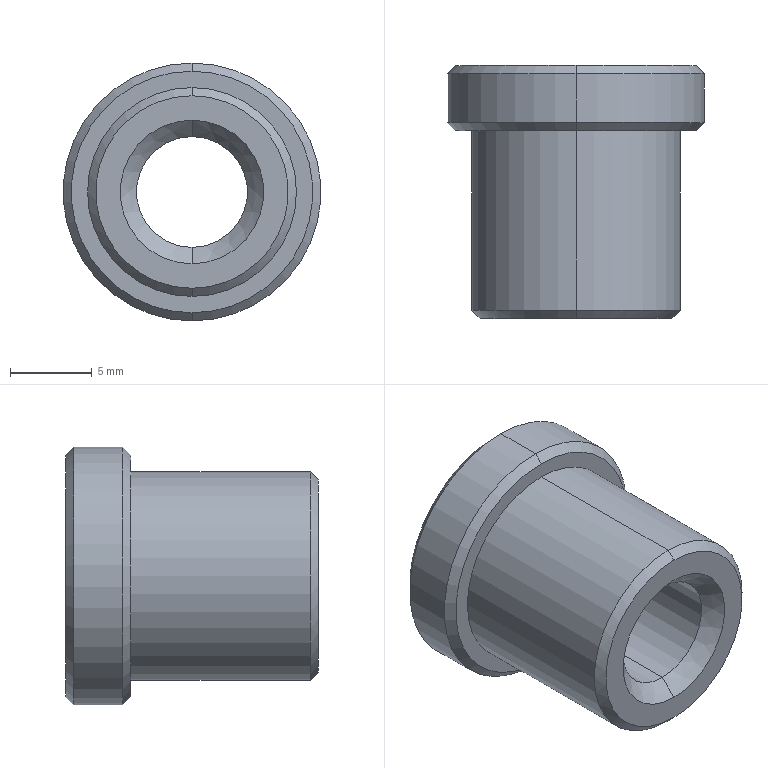Part | STEP file | CA-10-019Floating Joint | 1 solid | 19 faces | box 15.8 x 15.5 x 15.8 mm | volume 1661 mm3 | cone 10 | cylinder 6 | plane 3 | commonest cylinder face diameters 6.8 x2 12.8 x2 15.8 x2
STEP:
#1=CARTESIAN_POINT('',(0.,0.,0.));
#2=DIRECTION('',(0.,0.,1.));
#3=DIRECTION('',(1.,0.,0.));
#4=AXIS2_PLACEMENT_3D('',#1,#2,#3);
#5=CARTESIAN_POINT('',(0.,0.,-5.9));
#6=VERTEX_POINT('',#5);
#7=CARTESIAN_POINT('',(0.,0.,5.9));
#8=VERTEX_POINT('',#7);
#9=CARTESIAN_POINT('',(0.,0.,0.));
#10=DIRECTION('',(0.,-1.,0.));
#11=DIRECTION('',(0.,0.,-1.));
#12=AXIS2_PLACEMENT_3D('',#9,#10,#11);
#13=CIRCLE('',#12,5.9);
#14=CARTESIAN_POINT('',(0.,0.5,0.));
#15=DIRECTION('',(0.,1.,0.));
#16=DIRECTION('',(0.,0.,1.));
#17=AXIS2_PLACEMENT_3D('',#14,#15,#16);
#18=CONICAL_SURFACE('',#17,6.4,0.7854);
#19=CARTESIAN_POINT('',(3.142,-0.5));
#20=DIRECTION('',(-1.,0.));
#21=VECTOR('',#20,1.);
#22=LINE('',#19,#21);
#23=(GEOMETRIC_REPRESENTATION_CONTEXT(2)PARAMETRIC_REPRESENTATION_CONTEXT()REPRESENTATION_CONTEXT('',''));
#24=DEFINITIONAL_REPRESENTATION('',(#22),#23);
#25=PCURVE('',#18,#24);
#26=CARTESIAN_POINT('',(-2.5,0.,0.));
#27=DIRECTION('',(0.,-1.,0.));
#28=DIRECTION('',(0.,0.,-1.));
#29=AXIS2_PLACEMENT_3D('',#26,#27,#28);
#30=PLANE('',#29);
#31=CARTESIAN_POINT('',(0.,2.5));
#32=DIRECTION('',(1.,0.));
#33=AXIS2_PLACEMENT_2D('',#31,#32);
#34=CIRCLE('',#33,5.9);
#35=(GEOMETRIC_REPRESENTATION_CONTEXT(2)PARAMETRIC_REPRESENTATION_CONTEXT()REPRESENTATION_CONTEXT('',''));
#36=DEFINITIONAL_REPRESENTATION('',(#34),#35);
#37=PCURVE('',#30,#36);
#38=SURFACE_CURVE('',#13,(#25,#37),.PCURVE_S1.);
#39=EDGE_CURVE('',#6,#8,#38,.T.);
#40=ORIENTED_EDGE('',*,*,#39,.F.);
#41=CARTESIAN_POINT('',(0.,0.5,-6.4));
#42=VERTEX_POINT('',#41);
#43=CARTESIAN_POINT('',(0.,0.5,-6.4));
#44=DIRECTION('',(0.,0.7071,-0.7071));
#45=VECTOR('',#44,1.);
#46=LINE('',#43,#45);
#47=CARTESIAN_POINT('',(3.142,0.));
#48=DIRECTION('',(0.,1.));
#49=VECTOR('',#48,1.);
#50=LINE('',#47,#49);
#51=(GEOMETRIC_REPRESENTATION_CONTEXT(2)PARAMETRIC_REPRESENTATION_CONTEXT()REPRESENTATION_CONTEXT('',''));
#52=DEFINITIONAL_REPRESENTATION('',(#50),#51);
#53=PCURVE('',#18,#52);
#54=CARTESIAN_POINT('',(0.,0.5,0.));
#55=DIRECTION('',(0.,1.,0.));
#56=DIRECTION('',(0.,0.,1.));
#57=AXIS2_PLACEMENT_3D('',#54,#55,#56);
#58=CONICAL_SURFACE('',#57,6.4,0.7854);
#59=CARTESIAN_POINT('',(3.142,0.));
#60=DIRECTION('',(0.,1.));
#61=VECTOR('',#60,1.);
#62=LINE('',#59,#61);
#63=(GEOMETRIC_REPRESENTATION_CONTEXT(2)PARAMETRIC_REPRESENTATION_CONTEXT()REPRESENTATION_CONTEXT('',''));
#64=DEFINITIONAL_REPRESENTATION('',(#62),#63);
#65=PCURVE('',#58,#64);
#66=SURFACE_CURVE('',#46,(#53,#65),.PCURVE_S1.);
#67=EDGE_CURVE('',#6,#42,#66,.T.);
#68=ORIENTED_EDGE('',*,*,#67,.T.);
#69=CARTESIAN_POINT('',(0.,0.5,6.4));
#70=VERTEX_POINT('',#69);
#71=CARTESIAN_POINT('',(0.,0.5,0.));
#72=DIRECTION('',(0.,1.,0.));
#73=DIRECTION('',(0.,0.,-1.));
#74=AXIS2_PLACEMENT_3D('',#71,#72,#73);
#75=CIRCLE('',#74,6.4);
#76=CARTESIAN_POINT('',(-3.142,0.));
#77=DIRECTION('',(1.,0.));
#78=VECTOR('',#77,1.);
#79=LINE('',#76,#78);
#80=(GEOMETRIC_REPRESENTATION_CONTEXT(2)PARAMETRIC_REPRESENTATION_CONTEXT()REPRESENTATION_CONTEXT('',''));
#81=DEFINITIONAL_REPRESENTATION('',(#79),#80);
#82=PCURVE('',#18,#81);
#83=CARTESIAN_POINT('',(0.,-2.167,0.));
#84=DIRECTION('',(0.,1.,0.));
#85=DIRECTION('',(0.,0.,1.));
#86=AXIS2_PLACEMENT_3D('',#83,#84,#85);
#87=CYLINDRICAL_SURFACE('',#86,6.4);
#88=CARTESIAN_POINT('',(-3.142,2.667));
#89=DIRECTION('',(1.,0.));
#90=VECTOR('',#89,1.);
#91=LINE('',#88,#90);
#92=(GEOMETRIC_REPRESENTATION_CONTEXT(2)PARAMETRIC_REPRESENTATION_CONTEXT()REPRESENTATION_CONTEXT('',''));
#93=DEFINITIONAL_REPRESENTATION('',(#91),#92);
#94=PCURVE('',#87,#93);
#95=SURFACE_CURVE('',#75,(#82,#94),.PCURVE_S1.);
#96=EDGE_CURVE('',#70,#42,#95,.T.);
#97=ORIENTED_EDGE('',*,*,#96,.F.);
#98=CARTESIAN_POINT('',(0.,0.5,6.4));
#99=DIRECTION('',(0.,0.7071,0.7071));
#100=VECTOR('',#99,1.);
#101=LINE('',#98,#100);
#102=CARTESIAN_POINT('',(0.,0.));
#103=DIRECTION('',(0.,1.));
#104=VECTOR('',#103,1.);
#105=LINE('',#102,#104);
#106=(GEOMETRIC_REPRESENTATION_CONTEXT(2)PARAMETRIC_REPRESENTATION_CONTEXT()REPRESENTATION_CONTEXT('',''));
#107=DEFINITIONAL_REPRESENTATION('',(#105),#106);
#108=PCURVE('',#18,#107);
#109=CARTESIAN_POINT('',(6.283,0.));
#110=DIRECTION('',(0.,1.));
#111=VECTOR('',#110,1.);
#112=LINE('',#109,#111);
#113=(GEOMETRIC_REPRESENTATION_CONTEXT(2)PARAMETRIC_REPRESENTATION_CONTEXT()REPRESENTATION_CONTEXT('',''));
#114=DEFINITIONAL_REPRESENTATION('',(#112),#113);
#115=PCURVE('',#58,#114);
#116=SURFACE_CURVE('',#101,(#108,#115),.PCURVE_S1.);
#117=EDGE_CURVE('',#8,#70,#116,.T.);
#118=ORIENTED_EDGE('',*,*,#117,.F.);
#119=EDGE_LOOP('',(#40,#68,#97,#118));
#120=FACE_BOUND('',#119,.T.);
#121=ADVANCED_FACE('',(#120),#18,.T.);
#122=CARTESIAN_POINT('',(0.,11.5,-7.4));
#123=VERTEX_POINT('',#122);
#124=CARTESIAN_POINT('',(0.,11.5,7.4));
#125=VERTEX_POINT('',#124);
#126=CARTESIAN_POINT('',(0.,11.5,0.));
#127=DIRECTION('',(0.,-1.,0.));
#128=DIRECTION('',(0.,0.,-1.));
#129=AXIS2_PLACEMENT_3D('',#126,#127,#128);
#130=CIRCLE('',#129,7.4);
#131=CARTESIAN_POINT('',(0.,12.,0.));
#132=DIRECTION('',(0.,1.,0.));
#133=DIRECTION('',(0.,0.,1.));
#134=AXIS2_PLACEMENT_3D('',#131,#132,#133);
#135=CONICAL_SURFACE('',#134,7.9,0.7854);
#136=CARTESIAN_POINT('',(3.142,-0.5));
#137=DIRECTION('',(-1.,0.));
#138=VECTOR('',#137,1.);
#139=LINE('',#136,#138);
#140=(GEOMETRIC_REPRESENTATION_CONTEXT(2)PARAMETRIC_REPRESENTATION_CONTEXT()REPRESENTATION_CONTEXT('',''));
#141=DEFINITIONAL_REPRESENTATION('',(#139),#140);
#142=PCURVE('',#135,#141);
#143=CARTESIAN_POINT('',(-6.4,11.5,0.));
#144=DIRECTION('',(0.,-1.,0.));
#145=DIRECTION('',(0.,0.,-1.));
#146=AXIS2_PLACEMENT_3D('',#143,#144,#145);
#147=PLANE('',#146);
#148=CARTESIAN_POINT('',(0.,6.4));
#149=DIRECTION('',(1.,0.));
#150=AXIS2_PLACEMENT_2D('',#148,#149);
#151=CIRCLE('',#150,7.4);
#152=(GEOMETRIC_REPRESENTATION_CONTEXT(2)PARAMETRIC_REPRESENTATION_CONTEXT()REPRESENTATION_CONTEXT('',''));
#153=DEFINITIONAL_REPRESENTATION('',(#151),#152);
#154=PCURVE('',#147,#153);
#155=SURFACE_CURVE('',#130,(#142,#154),.PCURVE_S1.);
#156=EDGE_CURVE('',#123,#125,#155,.T.);
#157=ORIENTED_EDGE('',*,*,#156,.F.);
#158=CARTESIAN_POINT('',(0.,12.,-7.9));
#159=VERTEX_POINT('',#158);
#160=CARTESIAN_POINT('',(0.,12.,-7.9));
#161=DIRECTION('',(0.,0.7071,-0.7071));
#162=VECTOR('',#161,1.);
#163=LINE('',#160,#162);
#164=CARTESIAN_POINT('',(3.142,0.));
#165=DIRECTION('',(0.,1.));
#166=VECTOR('',#165,1.);
#167=LINE('',#164,#166);
#168=(GEOMETRIC_REPRESENTATION_CONTEXT(2)PARAMETRIC_REPRESENTATION_CONTEXT()REPRESENTATION_CONTEXT('',''));
#169=DEFINITIONAL_REPRESENTATION('',(#167),#168);
#170=PCURVE('',#135,#169);
#171=CARTESIAN_POINT('',(0.,12.,0.));
#172=DIRECTION('',(0.,1.,0.));
#173=DIRECTION('',(0.,0.,1.));
#174=AXIS2_PLACEMENT_3D('',#171,#172,#173);
#175=CONICAL_SURFACE('',#174,7.9,0.7854);
#176=CARTESIAN_POINT('',(3.142,0.));
#177=DIRECTION('',(0.,1.));
#178=VECTOR('',#177,1.);
#179=LINE('',#176,#178);
#180=(GEOMETRIC_REPRESENTATION_CONTEXT(2)PARAMETRIC_REPRESENTATION_CONTEXT()REPRESENTATION_CONTEXT('',''));
#181=DEFINITIONAL_REPRESENTATION('',(#179),#180);
#182=PCURVE('',#175,#181);
#183=SURFACE_CURVE('',#163,(#170,#182),.PCURVE_S1.);
#184=EDGE_CURVE('',#123,#159,#183,.T.);
#185=ORIENTED_EDGE('',*,*,#184,.T.);
#186=CARTESIAN_POINT('',(0.,12.,7.9));
#187=VERTEX_POINT('',#186);
#188=CARTESIAN_POINT('',(0.,12.,0.));
#189=DIRECTION('',(0.,1.,0.));
#190=DIRECTION('',(0.,0.,-1.));
#191=AXIS2_PLACEMENT_3D('',#188,#189,#190);
#192=CIRCLE('',#191,7.9);
#193=CARTESIAN_POINT('',(-3.142,0.));
#194=DIRECTION('',(1.,0.));
#195=VECTOR('',#194,1.);
#196=LINE('',#193,#195);
#197=(GEOMETRIC_REPRESENTATION_CONTEXT(2)PARAMETRIC_REPRESENTATION_CONTEXT()REPRESENTATION_CONTEXT('',''));
#198=DEFINITIONAL_REPRESENTATION('',(#196),#197);
#199=PCURVE('',#135,#198);
#200=CARTESIAN_POINT('',(0.,-2.167,0.));
#201=DIRECTION('',(0.,1.,0.));
#202=DIRECTION('',(0.,0.,1.));
#203=AXIS2_PLACEMENT_3D('',#200,#201,#202);
#204=CYLINDRICAL_SURFACE('',#203,7.9);
#205=CARTESIAN_POINT('',(-3.142,14.167));
#206=DIRECTION('',(1.,0.));
#207=VECTOR('',#206,1.);
#208=LINE('',#205,#207);
#209=(GEOMETRIC_REPRESENTATION_CONTEXT(2)PARAMETRIC_REPRESENTATION_CONTEXT()REPRESENTATION_CONTEXT('',''));
#210=DEFINITIONAL_REPRESENTATION('',(#208),#209);
#211=PCURVE('',#204,#210);
#212=SURFACE_CURVE('',#192,(#199,#211),.PCURVE_S1.);
#213=EDGE_CURVE('',#187,#159,#212,.T.);
#214=ORIENTED_EDGE('',*,*,#213,.F.);
#215=CARTESIAN_POINT('',(0.,12.,7.9));
#216=DIRECTION('',(0.,0.7071,0.7071));
#217=VECTOR('',#216,1.);
#218=LINE('',#215,#217);
#219=CARTESIAN_POINT('',(0.,0.));
#220=DIRECTION('',(0.,1.));
#221=VECTOR('',#220,1.);
#222=LINE('',#219,#221);
#223=(GEOMETRIC_REPRESENTATION_CONTEXT(2)PARAMETRIC_REPRESENTATION_CONTEXT()REPRESENTATION_CONTEXT('',''));
#224=DEFINITIONAL_REPRESENTATION('',(#222),#223);
#225=PCURVE('',#135,#224);
#226=CARTESIAN_POINT('',(6.283,0.));
#227=DIRECTION('',(0.,1.));
#228=VECTOR('',#227,1.);
#229=LINE('',#226,#228);
#230=(GEOMETRIC_REPRESENTATION_CONTEXT(2)PARAMETRIC_REPRESENTATION_CONTEXT()REPRESENTATION_CONTEXT('',''));
#231=DEFINITIONAL_REPRESENTATION('',(#229),#230);
#232=PCURVE('',#175,#231);
#233=SURFACE_CURVE('',#218,(#225,#232),.PCURVE_S1.);
#234=EDGE_CURVE('',#125,#187,#233,.T.);
#235=ORIENTED_EDGE('',*,*,#234,.F.);
#236=EDGE_LOOP('',(#157,#185,#214,#235));
#237=FACE_BOUND('',#236,.T.);
#238=ADVANCED_FACE('',(#237),#135,.T.);
#239=CARTESIAN_POINT('',(0.,15.5,7.4));
#240=VERTEX_POINT('',#239);
#241=CARTESIAN_POINT('',(0.,15.5,-7.4));
#242=VERTEX_POINT('',#241);
#243=CARTESIAN_POINT('',(0.,15.5,0.));
#244=DIRECTION('',(0.,1.,0.));
#245=DIRECTION('',(0.,0.,1.));
#246=AXIS2_PLACEMENT_3D('',#243,#244,#245);
#247=CIRCLE('',#246,7.4);
#248=CARTESIAN_POINT('',(0.,15.5,0.));
#249=DIRECTION('',(0.,-1.,0.));
#250=DIRECTION('',(0.,0.,-1.));
#251=AXIS2_PLACEMENT_3D('',#248,#249,#250);
#252=CONICAL_SURFACE('',#251,7.4,0.7854);
#253=CARTESIAN_POINT('',(3.142,0.));
#254=DIRECTION('',(-1.,0.));
#255=VECTOR('',#254,1.);
#256=LINE('',#253,#255);
#257=(GEOMETRIC_REPRESENTATION_CONTEXT(2)PARAMETRIC_REPRESENTATION_CONTEXT()REPRESENTATION_CONTEXT('',''));
#258=DEFINITIONAL_REPRESENTATION('',(#256),#257);
#259=PCURVE('',#252,#258);
#260=CARTESIAN_POINT('',(-7.9,15.5,0.));
#261=DIRECTION('',(0.,1.,0.));
#262=DIRECTION('',(0.,0.,1.));
#263=AXIS2_PLACEMENT_3D('',#260,#261,#262);
#264=PLANE('',#263);
#265=CARTESIAN_POINT('',(0.,7.9));
#266=DIRECTION('',(1.,0.));
#267=AXIS2_PLACEMENT_2D('',#265,#266);
#268=CIRCLE('',#267,7.4);
#269=(GEOMETRIC_REPRESENTATION_CONTEXT(2)PARAMETRIC_REPRESENTATION_CONTEXT()REPRESENTATION_CONTEXT('',''));
#270=DEFINITIONAL_REPRESENTATION('',(#268),#269);
#271=PCURVE('',#264,#270);
#272=SURFACE_CURVE('',#247,(#259,#271),.PCURVE_S1.);
#273=EDGE_CURVE('',#240,#242,#272,.T.);
#274=ORIENTED_EDGE('',*,*,#273,.F.);
#275=CARTESIAN_POINT('',(0.,15.,7.9));
#276=VERTEX_POINT('',#275);
#277=CARTESIAN_POINT('',(0.,15.5,7.4));
#278=DIRECTION('',(0.,-0.7071,0.7071));
#279=VECTOR('',#278,1.);
#280=LINE('',#277,#279);
#281=CARTESIAN_POINT('',(3.142,0.));
#282=DIRECTION('',(0.,1.));
#283=VECTOR('',#282,1.);
#284=LINE('',#281,#283);
#285=(GEOMETRIC_REPRESENTATION_CONTEXT(2)PARAMETRIC_REPRESENTATION_CONTEXT()REPRESENTATION_CONTEXT('',''));
#286=DEFINITIONAL_REPRESENTATION('',(#284),#285);
#287=PCURVE('',#252,#286);
#288=CARTESIAN_POINT('',(0.,15.5,0.));
#289=DIRECTION('',(0.,-1.,0.));
#290=DIRECTION('',(0.,0.,-1.));
#291=AXIS2_PLACEMENT_3D('',#288,#289,#290);
#292=CONICAL_SURFACE('',#291,7.4,0.7854);
#293=CARTESIAN_POINT('',(3.142,0.));
#294=DIRECTION('',(0.,1.));
#295=VECTOR('',#294,1.);
#296=LINE('',#293,#295);
#297=(GEOMETRIC_REPRESENTATION_CONTEXT(2)PARAMETRIC_REPRESENTATION_CONTEXT()REPRESENTATION_CONTEXT('',''));
#298=DEFINITIONAL_REPRESENTATION('',(#296),#297);
#299=PCURVE('',#292,#298);
#300=SURFACE_CURVE('',#280,(#287,#299),.PCURVE_S1.);
#301=EDGE_CURVE('',#240,#276,#300,.T.);
#302=ORIENTED_EDGE('',*,*,#301,.T.);
#303=CARTESIAN_POINT('',(0.,15.,-7.9));
#304=VERTEX_POINT('',#303);
#305=CARTESIAN_POINT('',(0.,15.,0.));
#306=DIRECTION('',(0.,-1.,0.));
#307=DIRECTION('',(0.,0.,1.));
#308=AXIS2_PLACEMENT_3D('',#305,#306,#307);
#309=CIRCLE('',#308,7.9);
#310=CARTESIAN_POINT('',(-3.142,0.5));
#311=DIRECTION('',(1.,0.));
#312=VECTOR('',#311,1.);
#313=LINE('',#310,#312);
#314=(GEOMETRIC_REPRESENTATION_CONTEXT(2)PARAMETRIC_REPRESENTATION_CONTEXT()REPRESENTATION_CONTEXT('',''));
#315=DEFINITIONAL_REPRESENTATION('',(#313),#314);
#316=PCURVE('',#252,#315);
#317=CARTESIAN_POINT('',(6.283,17.167));
#318=DIRECTION('',(-1.,0.));
#319=VECTOR('',#318,1.);
#320=LINE('',#317,#319);
#321=(GEOMETRIC_REPRESENTATION_CONTEXT(2)PARAMETRIC_REPRESENTATION_CONTEXT()REPRESENTATION_CONTEXT('',''));
#322=DEFINITIONAL_REPRESENTATION('',(#320),#321);
#323=PCURVE('',#204,#322);
#324=SURFACE_CURVE('',#309,(#316,#323),.PCURVE_S1.);
#325=EDGE_CURVE('',#304,#276,#324,.T.);
#326=ORIENTED_EDGE('',*,*,#325,.F.);
#327=CARTESIAN_POINT('',(0.,15.5,-7.4));
#328=DIRECTION('',(0.,-0.7071,-0.7071));
#329=VECTOR('',#328,1.);
#330=LINE('',#327,#329);
#331=CARTESIAN_POINT('',(0.,0.));
#332=DIRECTION('',(0.,1.));
#333=VECTOR('',#332,1.);
#334=LINE('',#331,#333);
#335=(GEOMETRIC_REPRESENTATION_CONTEXT(2)PARAMETRIC_REPRESENTATION_CONTEXT()REPRESENTATION_CONTEXT('',''));
#336=DEFINITIONAL_REPRESENTATION('',(#334),#335);
#337=PCURVE('',#252,#336);
#338=CARTESIAN_POINT('',(6.283,0.));
#339=DIRECTION('',(0.,1.));
#340=VECTOR('',#339,1.);
#341=LINE('',#338,#340);
#342=(GEOMETRIC_REPRESENTATION_CONTEXT(2)PARAMETRIC_REPRESENTATION_CONTEXT()REPRESENTATION_CONTEXT('',''));
#343=DEFINITIONAL_REPRESENTATION('',(#341),#342);
#344=PCURVE('',#292,#343);
#345=SURFACE_CURVE('',#330,(#337,#344),.PCURVE_S1.);
#346=EDGE_CURVE('',#242,#304,#345,.T.);
#347=ORIENTED_EDGE('',*,*,#346,.F.);
#348=EDGE_LOOP('',(#274,#302,#326,#347));
#349=FACE_BOUND('',#348,.T.);
#350=ADVANCED_FACE('',(#349),#252,.T.);
#351=CARTESIAN_POINT('',(0.,14.5,3.4));
#352=VERTEX_POINT('',#351);
#353=CARTESIAN_POINT('',(0.,15.5,4.4));
#354=VERTEX_POINT('',#353);
#355=CARTESIAN_POINT('',(0.,15.5,4.4));
#356=DIRECTION('',(0.,0.7071,0.7071));
#357=VECTOR('',#356,1.);
#358=LINE('',#355,#357);
#359=CARTESIAN_POINT('',(0.,15.5,0.));
#360=DIRECTION('',(0.,1.,0.));
#361=DIRECTION('',(0.,0.,1.));
#362=AXIS2_PLACEMENT_3D('',#359,#360,#361);
#363=CONICAL_SURFACE('',#362,4.4,0.7854);
#364=CARTESIAN_POINT('',(6.283,0.));
#365=DIRECTION('',(0.,1.));
#366=VECTOR('',#365,1.);
#367=LINE('',#364,#366);
#368=(GEOMETRIC_REPRESENTATION_CONTEXT(2)PARAMETRIC_REPRESENTATION_CONTEXT()REPRESENTATION_CONTEXT('',''));
#369=DEFINITIONAL_REPRESENTATION('',(#367),#368);
#370=PCURVE('',#363,#369);
#371=CARTESIAN_POINT('',(0.,15.5,0.));
#372=DIRECTION('',(0.,1.,0.));
#373=DIRECTION('',(0.,0.,1.));
#374=AXIS2_PLACEMENT_3D('',#371,#372,#373);
#375=CONICAL_SURFACE('',#374,4.4,0.7854);
#376=CARTESIAN_POINT('',(0.,0.));
#377=DIRECTION('',(0.,1.));
#378=VECTOR('',#377,1.);
#379=LINE('',#376,#378);
#380=(GEOMETRIC_REPRESENTATION_CONTEXT(2)PARAMETRIC_REPRESENTATION_CONTEXT()REPRESENTATION_CONTEXT('',''));
#381=DEFINITIONAL_REPRESENTATION('',(#379),#380);
#382=PCURVE('',#375,#381);
#383=SURFACE_CURVE('',#358,(#370,#382),.PCURVE_S1.);
#384=EDGE_CURVE('',#352,#354,#383,.T.);
#385=ORIENTED_EDGE('',*,*,#384,.T.);
#386=CARTESIAN_POINT('',(0.,15.5,-4.4));
#387=VERTEX_POINT('',#386);
#388=CARTESIAN_POINT('',(0.,15.5,0.));
#389=DIRECTION('',(0.,-1.,0.));
#390=DIRECTION('',(0.,0.,1.));
#391=AXIS2_PLACEMENT_3D('',#388,#389,#390);
#392=CIRCLE('',#391,4.4);
#393=CARTESIAN_POINT('',(6.283,0.));
#394=DIRECTION('',(-1.,0.));
#395=VECTOR('',#394,1.);
#396=LINE('',#393,#395);
#397=(GEOMETRIC_REPRESENTATION_CONTEXT(2)PARAMETRIC_REPRESENTATION_CONTEXT()REPRESENTATION_CONTEXT('',''));
#398=DEFINITIONAL_REPRESENTATION('',(#396),#397);
#399=PCURVE('',#363,#398);
#400=CARTESIAN_POINT('',(4.4,7.9));
#401=CARTESIAN_POINT('',(4.4,0.279));
#402=CARTESIAN_POINT('',(-2.2,4.089));
#403=CARTESIAN_POINT('',(-8.8,7.9));
#404=CARTESIAN_POINT('',(-2.2,11.711));
#405=CARTESIAN_POINT('',(4.4,15.521));
#406=CARTESIAN_POINT('',(4.4,7.9));
#407=(BOUNDED_CURVE()B_SPLINE_CURVE(2,(#400,#401,#402,#403,#404,#405,#406),.UNSPECIFIED.,.T.,.F.)B_SPLINE_CURVE_WITH_KNOTS((1,2,2,2,2,1),(-2.094,0.,2.094,4.189,6.283,8.378),.UNSPECIFIED.)CURVE()GEOMETRIC_REPRESENTATION_ITEM()RATIONAL_B_SPLINE_CURVE((1.,0.5,1.,0.5,1.,0.5,1.))REPRESENTATION_ITEM(''));
#408=(GEOMETRIC_REPRESENTATION_CONTEXT(2)PARAMETRIC_REPRESENTATION_CONTEXT()REPRESENTATION_CONTEXT('',''));
#409=DEFINITIONAL_REPRESENTATION('',(#407),#408);
#410=PCURVE('',#264,#409);
#411=SURFACE_CURVE('',#392,(#399,#410),.PCURVE_S1.);
#412=EDGE_CURVE('',#354,#387,#411,.T.);
#413=ORIENTED_EDGE('',*,*,#412,.T.);
#414=CARTESIAN_POINT('',(0.,14.5,-3.4));
#415=VERTEX_POINT('',#414);
#416=CARTESIAN_POINT('',(0.,15.5,-4.4));
#417=DIRECTION('',(0.,0.7071,-0.7071));
#418=VECTOR('',#417,1.);
#419=LINE('',#416,#418);
#420=CARTESIAN_POINT('',(3.142,0.));
#421=DIRECTION('',(0.,1.));
#422=VECTOR('',#421,1.);
#423=LINE('',#420,#422);
#424=(GEOMETRIC_REPRESENTATION_CONTEXT(2)PARAMETRIC_REPRESENTATION_CONTEXT()REPRESENTATION_CONTEXT('',''));
#425=DEFINITIONAL_REPRESENTATION('',(#423),#424);
#426=PCURVE('',#363,#425);
#427=CARTESIAN_POINT('',(3.142,0.));
#428=DIRECTION('',(0.,1.));
#429=VECTOR('',#428,1.);
#430=LINE('',#427,#429);
#431=(GEOMETRIC_REPRESENTATION_CONTEXT(2)PARAMETRIC_REPRESENTATION_CONTEXT()REPRESENTATION_CONTEXT('',''));
#432=DEFINITIONAL_REPRESENTATION('',(#430),#431);
#433=PCURVE('',#375,#432);
#434=SURFACE_CURVE('',#419,(#426,#433),.PCURVE_S1.);
#435=EDGE_CURVE('',#415,#387,#434,.T.);
#436=ORIENTED_EDGE('',*,*,#435,.F.);
#437=CARTESIAN_POINT('',(0.,14.5,0.));
#438=DIRECTION('',(0.,1.,0.));
#439=DIRECTION('',(0.,0.,1.));
#440=AXIS2_PLACEMENT_3D('',#437,#438,#439);
#441=CIRCLE('',#440,3.4);
#442=CARTESIAN_POINT('',(0.,-1.));
#443=DIRECTION('',(1.,0.));
#444=VECTOR('',#443,1.);
#445=LINE('',#442,#444);
#446=(GEOMETRIC_REPRESENTATION_CONTEXT(2)PARAMETRIC_REPRESENTATION_CONTEXT()REPRESENTATION_CONTEXT('',''));
#447=DEFINITIONAL_REPRESENTATION('',(#445),#446);
#448=PCURVE('',#363,#447);
#449=CARTESIAN_POINT('',(0.,0.,0.));
#450=DIRECTION('',(0.,-1.,0.));
#451=DIRECTION('',(0.,0.,-1.));
#452=AXIS2_PLACEMENT_3D('',#449,#450,#451);
#453=CYLINDRICAL_SURFACE('',#452,3.4);
#454=CARTESIAN_POINT('',(9.425,-14.5));
#455=DIRECTION('',(-1.,0.));
#456=VECTOR('',#455,1.);
#457=LINE('',#454,#456);
#458=(GEOMETRIC_REPRESENTATION_CONTEXT(2)PARAMETRIC_REPRESENTATION_CONTEXT()REPRESENTATION_CONTEXT('',''));
#459=DEFINITIONAL_REPRESENTATION('',(#457),#458);
#460=PCURVE('',#453,#459);
#461=SURFACE_CURVE('',#441,(#448,#460),.PCURVE_S1.);
#462=EDGE_CURVE('',#415,#352,#461,.T.);
#463=ORIENTED_EDGE('',*,*,#462,.T.);
#464=EDGE_LOOP('',(#385,#413,#436,#463));
#465=FACE_BOUND('',#464,.F.);
#466=ADVANCED_FACE('',(#465),#363,.F.);
#467=CARTESIAN_POINT('',(0.,1.,-3.4));
#468=VERTEX_POINT('',#467);
#469=CARTESIAN_POINT('',(0.,0.,-4.4));
#470=VERTEX_POINT('',#469);
#471=CARTESIAN_POINT('',(0.,1.,-3.4));
#472=DIRECTION('',(0.,-0.7071,-0.7071));
#473=VECTOR('',#472,1.);
#474=LINE('',#471,#473);
#475=CARTESIAN_POINT('',(0.,1.,0.));
#476=DIRECTION('',(0.,-1.,0.));
#477=DIRECTION('',(0.,0.,-1.));
#478=AXIS2_PLACEMENT_3D('',#475,#476,#477);
#479=CONICAL_SURFACE('',#478,3.4,0.7854);
#480=CARTESIAN_POINT('',(6.283,0.));
#481=DIRECTION('',(0.,1.));
#482=VECTOR('',#481,1.);
#483=LINE('',#480,#482);
#484=(GEOMETRIC_REPRESENTATION_CONTEXT(2)PARAMETRIC_REPRESENTATION_CONTEXT()REPRESENTATION_CONTEXT('',''));
#485=DEFINITIONAL_REPRESENTATION('',(#483),#484);
#486=PCURVE('',#479,#485);
#487=CARTESIAN_POINT('',(0.,1.,0.));
#488=DIRECTION('',(0.,-1.,0.));
#489=DIRECTION('',(0.,0.,-1.));
#490=AXIS2_PLACEMENT_3D('',#487,#488,#489);
#491=CONICAL_SURFACE('',#490,3.4,0.7854);
#492=CARTESIAN_POINT('',(0.,0.));
#493=DIRECTION('',(0.,1.));
#494=VECTOR('',#493,1.);
#495=LINE('',#492,#494);
#496=(GEOMETRIC_REPRESENTATION_CONTEXT(2)PARAMETRIC_REPRESENTATION_CONTEXT()REPRESENTATION_CONTEXT('',''));
#497=DEFINITIONAL_REPRESENTATION('',(#495),#496);
#498=PCURVE('',#491,#497);
#499=SURFACE_CURVE('',#474,(#486,#498),.PCURVE_S1.);
#500=EDGE_CURVE('',#468,#470,#499,.T.);
#501=ORIENTED_EDGE('',*,*,#500,.T.);
#502=CARTESIAN_POINT('',(0.,0.,4.4));
#503=VERTEX_POINT('',#502);
#504=CARTESIAN_POINT('',(0.,0.,0.));
#505=DIRECTION('',(0.,1.,0.));
#506=DIRECTION('',(0.,0.,-1.));
#507=AXIS2_PLACEMENT_3D('',#504,#505,#506);
#508=CIRCLE('',#507,4.4);
#509=CARTESIAN_POINT('',(6.283,1.));
#510=DIRECTION('',(-1.,0.));
#511=VECTOR('',#510,1.);
#512=LINE('',#509,#511);
#513=(GEOMETRIC_REPRESENTATION_CONTEXT(2)PARAMETRIC_REPRESENTATION_CONTEXT()REPRESENTATION_CONTEXT('',''));
#514=DEFINITIONAL_REPRESENTATION('',(#512),#513);
#515=PCURVE('',#479,#514);
#516=CARTESIAN_POINT('',(4.4,2.5));
#517=CARTESIAN_POINT('',(4.4,-5.121));
#518=CARTESIAN_POINT('',(-2.2,-1.311));
#519=CARTESIAN_POINT('',(-8.8,2.5));
#520=CARTESIAN_POINT('',(-2.2,6.311));
#521=CARTESIAN_POINT('',(4.4,10.121));
#522=CARTESIAN_POINT('',(4.4,2.5));
#523=(BOUNDED_CURVE()B_SPLINE_CURVE(2,(#516,#517,#518,#519,#520,#521,#522),.UNSPECIFIED.,.T.,.F.)B_SPLINE_CURVE_WITH_KNOTS((1,2,2,2,2,1),(-2.094,0.,2.094,4.189,6.283,8.378),.UNSPECIFIED.)CURVE()GEOMETRIC_REPRESENTATION_ITEM()RATIONAL_B_SPLINE_CURVE((1.,0.5,1.,0.5,1.,0.5,1.))REPRESENTATION_ITEM(''));
#524=(GEOMETRIC_REPRESENTATION_CONTEXT(2)PARAMETRIC_REPRESENTATION_CONTEXT()REPRESENTATION_CONTEXT('',''));
#525=DEFINITIONAL_REPRESENTATION('',(#523),#524);
#526=PCURVE('',#30,#525);
#527=SURFACE_CURVE('',#508,(#515,#526),.PCURVE_S1.);
#528=EDGE_CURVE('',#470,#503,#527,.T.);
#529=ORIENTED_EDGE('',*,*,#528,.T.);
#530=CARTESIAN_POINT('',(0.,1.,3.4));
#531=VERTEX_POINT('',#530);
#532=CARTESIAN_POINT('',(0.,1.,3.4));
#533=DIRECTION('',(0.,-0.7071,0.7071));
#534=VECTOR('',#533,1.);
#535=LINE('',#532,#534);
#536=CARTESIAN_POINT('',(3.142,0.));
#537=DIRECTION('',(0.,1.));
#538=VECTOR('',#537,1.);
#539=LINE('',#536,#538);
#540=(GEOMETRIC_REPRESENTATION_CONTEXT(2)PARAMETRIC_REPRESENTATION_CONTEXT()REPRESENTATION_CONTEXT('',''));
#541=DEFINITIONAL_REPRESENTATION('',(#539),#540);
#542=PCURVE('',#479,#541);
#543=CARTESIAN_POINT('',(3.142,0.));
#544=DIRECTION('',(0.,1.));
#545=VECTOR('',#544,1.);
#546=LINE('',#543,#545);
#547=(GEOMETRIC_REPRESENTATION_CONTEXT(2)PARAMETRIC_REPRESENTATION_CONTEXT()REPRESENTATION_CONTEXT('',''));
#548=DEFINITIONAL_REPRESENTATION('',(#546),#547);
#549=PCURVE('',#491,#548);
#550=SURFACE_CURVE('',#535,(#542,#549),.PCURVE_S1.);
#551=EDGE_CURVE('',#531,#503,#550,.T.);
#552=ORIENTED_EDGE('',*,*,#551,.F.);
#553=CARTESIAN_POINT('',(0.,1.,0.));
#554=DIRECTION('',(0.,-1.,0.));
#555=DIRECTION('',(0.,0.,-1.));
#556=AXIS2_PLACEMENT_3D('',#553,#554,#555);
#557=CIRCLE('',#556,3.4);
#558=CARTESIAN_POINT('',(0.,0.));
#559=DIRECTION('',(1.,0.));
#560=VECTOR('',#559,1.);
#561=LINE('',#558,#560);
#562=(GEOMETRIC_REPRESENTATION_CONTEXT(2)PARAMETRIC_REPRESENTATION_CONTEXT()REPRESENTATION_CONTEXT('',''));
#563=DEFINITIONAL_REPRESENTATION('',(#561),#562);
#564=PCURVE('',#479,#563);
#565=CARTESIAN_POINT('',(0.,-1.));
#566=DIRECTION('',(1.,0.));
#567=VECTOR('',#566,1.);
#568=LINE('',#565,#567);
#569=(GEOMETRIC_REPRESENTATION_CONTEXT(2)PARAMETRIC_REPRESENTATION_CONTEXT()REPRESENTATION_CONTEXT('',''));
#570=DEFINITIONAL_REPRESENTATION('',(#568),#569);
#571=PCURVE('',#453,#570);
#572=SURFACE_CURVE('',#557,(#564,#571),.PCURVE_S1.);
#573=EDGE_CURVE('',#531,#468,#572,.T.);
#574=ORIENTED_EDGE('',*,*,#573,.T.);
#575=EDGE_LOOP('',(#501,#529,#552,#574));
#576=FACE_BOUND('',#575,.F.);
#577=ADVANCED_FACE('',(#576),#479,.F.);
#578=CARTESIAN_POINT('',(0.,0.,-3.4));
#579=DIRECTION('',(0.,-1.,0.));
#580=VECTOR('',#579,1.);
#581=LINE('',#578,#580);
#582=CARTESIAN_POINT('',(6.283,0.));
#583=DIRECTION('',(0.,1.));
#584=VECTOR('',#583,1.);
#585=LINE('',#582,#584);
#586=(GEOMETRIC_REPRESENTATION_CONTEXT(2)PARAMETRIC_REPRESENTATION_CONTEXT()REPRESENTATION_CONTEXT('',''));
#587=DEFINITIONAL_REPRESENTATION('',(#585),#586);
#588=PCURVE('',#453,#587);
#589=CARTESIAN_POINT('',(0.,0.,0.));
#590=DIRECTION('',(0.,-1.,0.));
#591=DIRECTION('',(0.,0.,-1.));
#592=AXIS2_PLACEMENT_3D('',#589,#590,#591);
#593=CYLINDRICAL_SURFACE('',#592,3.4);
#594=CARTESIAN_POINT('',(0.,0.));
#595=DIRECTION('',(0.,1.));
#596=VECTOR('',#595,1.);
#597=LINE('',#594,#596);
#598=(GEOMETRIC_REPRESENTATION_CONTEXT(2)PARAMETRIC_REPRESENTATION_CONTEXT()REPRESENTATION_CONTEXT('',''));
#599=DEFINITIONAL_REPRESENTATION('',(#597),#598);
#600=PCURVE('',#593,#599);
#601=SURFACE_CURVE('',#581,(#588,#600),.PCURVE_S1.);
#602=EDGE_CURVE('',#415,#468,#601,.T.);
#603=ORIENTED_EDGE('',*,*,#602,.T.);
#604=ORIENTED_EDGE('',*,*,#573,.F.);
#605=CARTESIAN_POINT('',(0.,0.,3.4));
#606=DIRECTION('',(0.,-1.,0.));
#607=VECTOR('',#606,1.);
#608=LINE('',#605,#607);
#609=CARTESIAN_POINT('',(3.142,0.));
#610=DIRECTION('',(0.,1.));
#611=VECTOR('',#610,1.);
#612=LINE('',#609,#611);
#613=(GEOMETRIC_REPRESENTATION_CONTEXT(2)PARAMETRIC_REPRESENTATION_CONTEXT()REPRESENTATION_CONTEXT('',''));
#614=DEFINITIONAL_REPRESENTATION('',(#612),#613);
#615=PCURVE('',#453,#614);
#616=CARTESIAN_POINT('',(3.142,0.));
#617=DIRECTION('',(0.,1.));
#618=VECTOR('',#617,1.);
#619=LINE('',#616,#618);
#620=(GEOMETRIC_REPRESENTATION_CONTEXT(2)PARAMETRIC_REPRESENTATION_CONTEXT()REPRESENTATION_CONTEXT('',''));
#621=DEFINITIONAL_REPRESENTATION('',(#619),#620);
#622=PCURVE('',#593,#621);
#623=SURFACE_CURVE('',#608,(#615,#622),.PCURVE_S1.);
#624=EDGE_CURVE('',#352,#531,#623,.T.);
#625=ORIENTED_EDGE('',*,*,#624,.F.);
#626=ORIENTED_EDGE('',*,*,#462,.F.);
#627=EDGE_LOOP('',(#603,#604,#625,#626));
#628=FACE_BOUND('',#627,.F.);
#629=ADVANCED_FACE('',(#628),#453,.F.);
#630=ORIENTED_EDGE('',*,*,#213,.T.);
#631=CARTESIAN_POINT('',(0.,-2.167,-7.9));
#632=DIRECTION('',(0.,1.,0.));
#633=VECTOR('',#632,1.);
#634=LINE('',#631,#633);
#635=CARTESIAN_POINT('',(3.142,0.));
#636=DIRECTION('',(0.,1.));
#637=VECTOR('',#636,1.);
#638=LINE('',#635,#637);
#639=(GEOMETRIC_REPRESENTATION_CONTEXT(2)PARAMETRIC_REPRESENTATION_CONTEXT()REPRESENTATION_CONTEXT('',''));
#640=DEFINITIONAL_REPRESENTATION('',(#638),#639);
#641=PCURVE('',#204,#640);
#642=CARTESIAN_POINT('',(0.,-2.167,0.));
#643=DIRECTION('',(0.,1.,0.));
#644=DIRECTION('',(0.,0.,1.));
#645=AXIS2_PLACEMENT_3D('',#642,#643,#644);
#646=CYLINDRICAL_SURFACE('',#645,7.9);
#647=CARTESIAN_POINT('',(3.142,0.));
#648=DIRECTION('',(0.,1.));
#649=VECTOR('',#648,1.);
#650=LINE('',#647,#649);
#651=(GEOMETRIC_REPRESENTATION_CONTEXT(2)PARAMETRIC_REPRESENTATION_CONTEXT()REPRESENTATION_CONTEXT('',''));
#652=DEFINITIONAL_REPRESENTATION('',(#650),#651);
#653=PCURVE('',#646,#652);
#654=SURFACE_CURVE('',#634,(#641,#653),.PCURVE_S1.);
#655=EDGE_CURVE('',#159,#304,#654,.T.);
#656=ORIENTED_EDGE('',*,*,#655,.T.);
#657=ORIENTED_EDGE('',*,*,#325,.T.);
#658=CARTESIAN_POINT('',(0.,-2.167,7.9));
#659=DIRECTION('',(0.,1.,0.));
#660=VECTOR('',#659,1.);
#661=LINE('',#658,#660);
#662=CARTESIAN_POINT('',(0.,0.));
#663=DIRECTION('',(0.,1.));
#664=VECTOR('',#663,1.);
#665=LINE('',#662,#664);
#666=(GEOMETRIC_REPRESENTATION_CONTEXT(2)PARAMETRIC_REPRESENTATION_CONTEXT()REPRESENTATION_CONTEXT('',''));
#667=DEFINITIONAL_REPRESENTATION('',(#665),#666);
#668=PCURVE('',#204,#667);
#669=CARTESIAN_POINT('',(6.283,0.));
#670=DIRECTION('',(0.,1.));
#671=VECTOR('',#670,1.);
#672=LINE('',#669,#671);
#673=(GEOMETRIC_REPRESENTATION_CONTEXT(2)PARAMETRIC_REPRESENTATION_CONTEXT()REPRESENTATION_CONTEXT('',''));
#674=DEFINITIONAL_REPRESENTATION('',(#672),#673);
#675=PCURVE('',#646,#674);
#676=SURFACE_CURVE('',#661,(#668,#675),.PCURVE_S1.);
#677=EDGE_CURVE('',#187,#276,#676,.T.);
#678=ORIENTED_EDGE('',*,*,#677,.F.);
#679=EDGE_LOOP('',(#630,#656,#657,#678));
#680=FACE_BOUND('',#679,.T.);
#681=ADVANCED_FACE('',(#680),#204,.T.);
#682=ORIENTED_EDGE('',*,*,#96,.T.);
#683=CARTESIAN_POINT('',(0.,11.5,-6.4));
#684=VERTEX_POINT('',#683);
#685=CARTESIAN_POINT('',(0.,-2.167,-6.4));
#686=DIRECTION('',(0.,1.,0.));
#687=VECTOR('',#686,1.);
#688=LINE('',#685,#687);
#689=CARTESIAN_POINT('',(3.142,0.));
#690=DIRECTION('',(0.,1.));
#691=VECTOR('',#690,1.);
#692=LINE('',#689,#691);
#693=(GEOMETRIC_REPRESENTATION_CONTEXT(2)PARAMETRIC_REPRESENTATION_CONTEXT()REPRESENTATION_CONTEXT('',''));
#694=DEFINITIONAL_REPRESENTATION('',(#692),#693);
#695=PCURVE('',#87,#694);
#696=CARTESIAN_POINT('',(0.,-2.167,0.));
#697=DIRECTION('',(0.,1.,0.));
#698=DIRECTION('',(0.,0.,1.));
#699=AXIS2_PLACEMENT_3D('',#696,#697,#698);
#700=CYLINDRICAL_SURFACE('',#699,6.4);
#701=CARTESIAN_POINT('',(3.142,0.));
#702=DIRECTION('',(0.,1.));
#703=VECTOR('',#702,1.);
#704=LINE('',#701,#703);
#705=(GEOMETRIC_REPRESENTATION_CONTEXT(2)PARAMETRIC_REPRESENTATION_CONTEXT()REPRESENTATION_CONTEXT('',''));
#706=DEFINITIONAL_REPRESENTATION('',(#704),#705);
#707=PCURVE('',#700,#706);
#708=SURFACE_CURVE('',#688,(#695,#707),.PCURVE_S1.);
#709=EDGE_CURVE('',#42,#684,#708,.T.);
#710=ORIENTED_EDGE('',*,*,#709,.T.);
#711=CARTESIAN_POINT('',(0.,11.5,6.4));
#712=VERTEX_POINT('',#711);
#713=CARTESIAN_POINT('',(0.,11.5,0.));
#714=DIRECTION('',(0.,1.,0.));
#715=DIRECTION('',(0.,0.,1.));
#716=AXIS2_PLACEMENT_3D('',#713,#714,#715);
#717=CIRCLE('',#716,6.4);
#718=CARTESIAN_POINT('',(0.,13.667));
#719=DIRECTION('',(1.,0.));
#720=VECTOR('',#719,1.);
#721=LINE('',#718,#720);
#722=(GEOMETRIC_REPRESENTATION_CONTEXT(2)PARAMETRIC_REPRESENTATION_CONTEXT()REPRESENTATION_CONTEXT('',''));
#723=DEFINITIONAL_REPRESENTATION('',(#721),#722);
#724=PCURVE('',#87,#723);
#725=CARTESIAN_POINT('',(-6.4,6.4));
#726=CARTESIAN_POINT('',(-6.4,17.485));
#727=CARTESIAN_POINT('',(3.2,11.943));
#728=CARTESIAN_POINT('',(12.8,6.4));
#729=CARTESIAN_POINT('',(3.2,0.8574));
#730=CARTESIAN_POINT('',(-6.4,-4.685));
#731=CARTESIAN_POINT('',(-6.4,6.4));
#732=(BOUNDED_CURVE()B_SPLINE_CURVE(2,(#725,#726,#727,#728,#729,#730,#731),.UNSPECIFIED.,.T.,.F.)B_SPLINE_CURVE_WITH_KNOTS((1,2,2,2,2,1),(-2.094,0.,2.094,4.189,6.283,8.378),.UNSPECIFIED.)CURVE()GEOMETRIC_REPRESENTATION_ITEM()RATIONAL_B_SPLINE_CURVE((1.,0.5,1.,0.5,1.,0.5,1.))REPRESENTATION_ITEM(''));
#733=(GEOMETRIC_REPRESENTATION_CONTEXT(2)PARAMETRIC_REPRESENTATION_CONTEXT()REPRESENTATION_CONTEXT('',''));
#734=DEFINITIONAL_REPRESENTATION('',(#732),#733);
#735=PCURVE('',#147,#734);
#736=SURFACE_CURVE('',#717,(#724,#735),.PCURVE_S1.);
#737=EDGE_CURVE('',#712,#684,#736,.T.);
#738=ORIENTED_EDGE('',*,*,#737,.F.);
#739=CARTESIAN_POINT('',(0.,-2.167,6.4));
#740=DIRECTION('',(0.,1.,0.));
#741=VECTOR('',#740,1.);
#742=LINE('',#739,#741);
#743=CARTESIAN_POINT('',(0.,0.));
#744=DIRECTION('',(0.,1.));
#745=VECTOR('',#744,1.);
#746=LINE('',#743,#745);
#747=(GEOMETRIC_REPRESENTATION_CONTEXT(2)PARAMETRIC_REPRESENTATION_CONTEXT()REPRESENTATION_CONTEXT('',''));
#748=DEFINITIONAL_REPRESENTATION('',(#746),#747);
#749=PCURVE('',#87,#748);
#750=CARTESIAN_POINT('',(6.283,0.));
#751=DIRECTION('',(0.,1.));
#752=VECTOR('',#751,1.);
#753=LINE('',#750,#752);
#754=(GEOMETRIC_REPRESENTATION_CONTEXT(2)PARAMETRIC_REPRESENTATION_CONTEXT()REPRESENTATION_CONTEXT('',''));
#755=DEFINITIONAL_REPRESENTATION('',(#753),#754);
#756=PCURVE('',#700,#755);
#757=SURFACE_CURVE('',#742,(#749,#756),.PCURVE_S1.);
#758=EDGE_CURVE('',#70,#712,#757,.T.);
#759=ORIENTED_EDGE('',*,*,#758,.F.);
#760=EDGE_LOOP('',(#682,#710,#738,#759));
#761=FACE_BOUND('',#760,.T.);
#762=ADVANCED_FACE('',(#761),#87,.T.);
#763=CARTESIAN_POINT('',(0.,0.,0.));
#764=DIRECTION('',(0.,-1.,0.));
#765=DIRECTION('',(0.,0.,-1.));
#766=AXIS2_PLACEMENT_3D('',#763,#764,#765);
#767=CIRCLE('',#766,5.9);
#768=CARTESIAN_POINT('',(0.,2.5));
#769=DIRECTION('',(1.,0.));
#770=AXIS2_PLACEMENT_2D('',#768,#769);
#771=CIRCLE('',#770,5.9);
#772=(GEOMETRIC_REPRESENTATION_CONTEXT(2)PARAMETRIC_REPRESENTATION_CONTEXT()REPRESENTATION_CONTEXT('',''));
#773=DEFINITIONAL_REPRESENTATION('',(#771),#772);
#774=PCURVE('',#30,#773);
#775=CARTESIAN_POINT('',(9.425,-0.5));
#776=DIRECTION('',(-1.,0.));
#777=VECTOR('',#776,1.);
#778=LINE('',#775,#777);
#779=(GEOMETRIC_REPRESENTATION_CONTEXT(2)PARAMETRIC_REPRESENTATION_CONTEXT()REPRESENTATION_CONTEXT('',''));
#780=DEFINITIONAL_REPRESENTATION('',(#778),#779);
#781=PCURVE('',#58,#780);
#782=SURFACE_CURVE('',#767,(#774,#781),.PCURVE_S1.);
#783=EDGE_CURVE('',#8,#6,#782,.T.);
#784=ORIENTED_EDGE('',*,*,#783,.T.);
#785=ORIENTED_EDGE('',*,*,#39,.T.);
#786=EDGE_LOOP('',(#784,#785));
#787=FACE_BOUND('',#786,.T.);
#788=ORIENTED_EDGE('',*,*,#528,.T.);
#789=CARTESIAN_POINT('',(0.,0.,0.));
#790=DIRECTION('',(0.,1.,0.));
#791=DIRECTION('',(0.,0.,-1.));
#792=AXIS2_PLACEMENT_3D('',#789,#790,#791);
#793=CIRCLE('',#792,4.4);
#794=CARTESIAN_POINT('',(4.4,2.5));
#795=CARTESIAN_POINT('',(4.4,-5.121));
#796=CARTESIAN_POINT('',(-2.2,-1.311));
#797=CARTESIAN_POINT('',(-8.8,2.5));
#798=CARTESIAN_POINT('',(-2.2,6.311));
#799=CARTESIAN_POINT('',(4.4,10.121));
#800=CARTESIAN_POINT('',(4.4,2.5));
#801=(BOUNDED_CURVE()B_SPLINE_CURVE(2,(#794,#795,#796,#797,#798,#799,#800),.UNSPECIFIED.,.T.,.F.)B_SPLINE_CURVE_WITH_KNOTS((1,2,2,2,2,1),(-2.094,0.,2.094,4.189,6.283,8.378),.UNSPECIFIED.)CURVE()GEOMETRIC_REPRESENTATION_ITEM()RATIONAL_B_SPLINE_CURVE((1.,0.5,1.,0.5,1.,0.5,1.))REPRESENTATION_ITEM(''));
#802=(GEOMETRIC_REPRESENTATION_CONTEXT(2)PARAMETRIC_REPRESENTATION_CONTEXT()REPRESENTATION_CONTEXT('',''));
#803=DEFINITIONAL_REPRESENTATION('',(#801),#802);
#804=PCURVE('',#30,#803);
#805=CARTESIAN_POINT('',(6.283,1.));
#806=DIRECTION('',(-1.,0.));
#807=VECTOR('',#806,1.);
#808=LINE('',#805,#807);
#809=(GEOMETRIC_REPRESENTATION_CONTEXT(2)PARAMETRIC_REPRESENTATION_CONTEXT()REPRESENTATION_CONTEXT('',''));
#810=DEFINITIONAL_REPRESENTATION('',(#808),#809);
#811=PCURVE('',#491,#810);
#812=SURFACE_CURVE('',#793,(#804,#811),.PCURVE_S1.);
#813=EDGE_CURVE('',#503,#470,#812,.T.);
#814=ORIENTED_EDGE('',*,*,#813,.T.);
#815=EDGE_LOOP('',(#788,#814));
#816=FACE_BOUND('',#815,.T.);
#817=ADVANCED_FACE('',(#787,#816),#30,.T.);
#818=ORIENTED_EDGE('',*,*,#709,.F.);
#819=CARTESIAN_POINT('',(0.,0.5,0.));
#820=DIRECTION('',(0.,1.,0.));
#821=DIRECTION('',(0.,0.,-1.));
#822=AXIS2_PLACEMENT_3D('',#819,#820,#821);
#823=CIRCLE('',#822,6.4);
#824=CARTESIAN_POINT('',(3.142,2.667));
#825=DIRECTION('',(1.,0.));
#826=VECTOR('',#825,1.);
#827=LINE('',#824,#826);
#828=(GEOMETRIC_REPRESENTATION_CONTEXT(2)PARAMETRIC_REPRESENTATION_CONTEXT()REPRESENTATION_CONTEXT('',''));
#829=DEFINITIONAL_REPRESENTATION('',(#827),#828);
#830=PCURVE('',#700,#829);
#831=CARTESIAN_POINT('',(3.142,0.));
#832=DIRECTION('',(1.,0.));
#833=VECTOR('',#832,1.);
#834=LINE('',#831,#833);
#835=(GEOMETRIC_REPRESENTATION_CONTEXT(2)PARAMETRIC_REPRESENTATION_CONTEXT()REPRESENTATION_CONTEXT('',''));
#836=DEFINITIONAL_REPRESENTATION('',(#834),#835);
#837=PCURVE('',#58,#836);
#838=SURFACE_CURVE('',#823,(#830,#837),.PCURVE_S1.);
#839=EDGE_CURVE('',#42,#70,#838,.T.);
#840=ORIENTED_EDGE('',*,*,#839,.T.);
#841=ORIENTED_EDGE('',*,*,#758,.T.);
#842=CARTESIAN_POINT('',(0.,11.5,0.));
#843=DIRECTION('',(0.,1.,0.));
#844=DIRECTION('',(0.,0.,1.));
#845=AXIS2_PLACEMENT_3D('',#842,#843,#844);
#846=CIRCLE('',#845,6.4);
#847=CARTESIAN_POINT('',(0.,13.667));
#848=DIRECTION('',(1.,0.));
#849=VECTOR('',#848,1.);
#850=LINE('',#847,#849);
#851=(GEOMETRIC_REPRESENTATION_CONTEXT(2)PARAMETRIC_REPRESENTATION_CONTEXT()REPRESENTATION_CONTEXT('',''));
#852=DEFINITIONAL_REPRESENTATION('',(#850),#851);
#853=PCURVE('',#700,#852);
#854=CARTESIAN_POINT('',(-6.4,6.4));
#855=CARTESIAN_POINT('',(-6.4,17.485));
#856=CARTESIAN_POINT('',(3.2,11.943));
#857=CARTESIAN_POINT('',(12.8,6.4));
#858=CARTESIAN_POINT('',(3.2,0.8574));
#859=CARTESIAN_POINT('',(-6.4,-4.685));
#860=CARTESIAN_POINT('',(-6.4,6.4));
#861=(BOUNDED_CURVE()B_SPLINE_CURVE(2,(#854,#855,#856,#857,#858,#859,#860),.UNSPECIFIED.,.T.,.F.)B_SPLINE_CURVE_WITH_KNOTS((1,2,2,2,2,1),(-2.094,0.,2.094,4.189,6.283,8.378),.UNSPECIFIED.)CURVE()GEOMETRIC_REPRESENTATION_ITEM()RATIONAL_B_SPLINE_CURVE((1.,0.5,1.,0.5,1.,0.5,1.))REPRESENTATION_ITEM(''));
#862=(GEOMETRIC_REPRESENTATION_CONTEXT(2)PARAMETRIC_REPRESENTATION_CONTEXT()REPRESENTATION_CONTEXT('',''));
#863=DEFINITIONAL_REPRESENTATION('',(#861),#862);
#864=PCURVE('',#147,#863);
#865=SURFACE_CURVE('',#846,(#853,#864),.PCURVE_S1.);
#866=EDGE_CURVE('',#684,#712,#865,.T.);
#867=ORIENTED_EDGE('',*,*,#866,.F.);
#868=EDGE_LOOP('',(#818,#840,#841,#867));
#869=FACE_BOUND('',#868,.T.);
#870=ADVANCED_FACE('',(#869),#700,.T.);
#871=CARTESIAN_POINT('',(0.,11.5,0.));
#872=DIRECTION('',(0.,-1.,0.));
#873=DIRECTION('',(0.,0.,-1.));
#874=AXIS2_PLACEMENT_3D('',#871,#872,#873);
#875=CIRCLE('',#874,7.4);
#876=CARTESIAN_POINT('',(0.,6.4));
#877=DIRECTION('',(1.,0.));
#878=AXIS2_PLACEMENT_2D('',#876,#877);
#879=CIRCLE('',#878,7.4);
#880=(GEOMETRIC_REPRESENTATION_CONTEXT(2)PARAMETRIC_REPRESENTATION_CONTEXT()REPRESENTATION_CONTEXT('',''));
#881=DEFINITIONAL_REPRESENTATION('',(#879),#880);
#882=PCURVE('',#147,#881);
#883=CARTESIAN_POINT('',(9.425,-0.5));
#884=DIRECTION('',(-1.,0.));
#885=VECTOR('',#884,1.);
#886=LINE('',#883,#885);
#887=(GEOMETRIC_REPRESENTATION_CONTEXT(2)PARAMETRIC_REPRESENTATION_CONTEXT()REPRESENTATION_CONTEXT('',''));
#888=DEFINITIONAL_REPRESENTATION('',(#886),#887);
#889=PCURVE('',#175,#888);
#890=SURFACE_CURVE('',#875,(#882,#889),.PCURVE_S1.);
#891=EDGE_CURVE('',#125,#123,#890,.T.);
#892=ORIENTED_EDGE('',*,*,#891,.T.);
#893=ORIENTED_EDGE('',*,*,#156,.T.);
#894=EDGE_LOOP('',(#892,#893));
#895=FACE_BOUND('',#894,.T.);
#896=ORIENTED_EDGE('',*,*,#737,.T.);
#897=ORIENTED_EDGE('',*,*,#866,.T.);
#898=EDGE_LOOP('',(#896,#897));
#899=FACE_BOUND('',#898,.T.);
#900=ADVANCED_FACE('',(#895,#899),#147,.T.);
#901=ORIENTED_EDGE('',*,*,#655,.F.);
#902=CARTESIAN_POINT('',(0.,12.,0.));
#903=DIRECTION('',(0.,1.,0.));
#904=DIRECTION('',(0.,0.,-1.));
#905=AXIS2_PLACEMENT_3D('',#902,#903,#904);
#906=CIRCLE('',#905,7.9);
#907=CARTESIAN_POINT('',(3.142,14.167));
#908=DIRECTION('',(1.,0.));
#909=VECTOR('',#908,1.);
#910=LINE('',#907,#909);
#911=(GEOMETRIC_REPRESENTATION_CONTEXT(2)PARAMETRIC_REPRESENTATION_CONTEXT()REPRESENTATION_CONTEXT('',''));
#912=DEFINITIONAL_REPRESENTATION('',(#910),#911);
#913=PCURVE('',#646,#912);
#914=CARTESIAN_POINT('',(3.142,0.));
#915=DIRECTION('',(1.,0.));
#916=VECTOR('',#915,1.);
#917=LINE('',#914,#916);
#918=(GEOMETRIC_REPRESENTATION_CONTEXT(2)PARAMETRIC_REPRESENTATION_CONTEXT()REPRESENTATION_CONTEXT('',''));
#919=DEFINITIONAL_REPRESENTATION('',(#917),#918);
#920=PCURVE('',#175,#919);
#921=SURFACE_CURVE('',#906,(#913,#920),.PCURVE_S1.);
#922=EDGE_CURVE('',#159,#187,#921,.T.);
#923=ORIENTED_EDGE('',*,*,#922,.T.);
#924=ORIENTED_EDGE('',*,*,#677,.T.);
#925=CARTESIAN_POINT('',(0.,15.,0.));
#926=DIRECTION('',(0.,-1.,0.));
#927=DIRECTION('',(0.,0.,1.));
#928=AXIS2_PLACEMENT_3D('',#925,#926,#927);
#929=CIRCLE('',#928,7.9);
#930=CARTESIAN_POINT('',(6.283,17.167));
#931=DIRECTION('',(-1.,0.));
#932=VECTOR('',#931,1.);
#933=LINE('',#930,#932);
#934=(GEOMETRIC_REPRESENTATION_CONTEXT(2)PARAMETRIC_REPRESENTATION_CONTEXT()REPRESENTATION_CONTEXT('',''));
#935=DEFINITIONAL_REPRESENTATION('',(#933),#934);
#936=PCURVE('',#646,#935);
#937=CARTESIAN_POINT('',(3.142,0.5));
#938=DIRECTION('',(1.,0.));
#939=VECTOR('',#938,1.);
#940=LINE('',#937,#939);
#941=(GEOMETRIC_REPRESENTATION_CONTEXT(2)PARAMETRIC_REPRESENTATION_CONTEXT()REPRESENTATION_CONTEXT('',''));
#942=DEFINITIONAL_REPRESENTATION('',(#940),#941);
#943=PCURVE('',#292,#942);
#944=SURFACE_CURVE('',#929,(#936,#943),.PCURVE_S1.);
#945=EDGE_CURVE('',#276,#304,#944,.T.);
#946=ORIENTED_EDGE('',*,*,#945,.T.);
#947=EDGE_LOOP('',(#901,#923,#924,#946));
#948=FACE_BOUND('',#947,.T.);
#949=ADVANCED_FACE('',(#948),#646,.T.);
#950=CARTESIAN_POINT('',(0.,15.5,0.));
#951=DIRECTION('',(0.,1.,0.));
#952=DIRECTION('',(0.,0.,1.));
#953=AXIS2_PLACEMENT_3D('',#950,#951,#952);
#954=CIRCLE('',#953,7.4);
#955=CARTESIAN_POINT('',(0.,7.9));
#956=DIRECTION('',(1.,0.));
#957=AXIS2_PLACEMENT_2D('',#955,#956);
#958=CIRCLE('',#957,7.4);
#959=(GEOMETRIC_REPRESENTATION_CONTEXT(2)PARAMETRIC_REPRESENTATION_CONTEXT()REPRESENTATION_CONTEXT('',''));
#960=DEFINITIONAL_REPRESENTATION('',(#958),#959);
#961=PCURVE('',#264,#960);
#962=CARTESIAN_POINT('',(9.425,0.));
#963=DIRECTION('',(-1.,0.));
#964=VECTOR('',#963,1.);
#965=LINE('',#962,#964);
#966=(GEOMETRIC_REPRESENTATION_CONTEXT(2)PARAMETRIC_REPRESENTATION_CONTEXT()REPRESENTATION_CONTEXT('',''));
#967=DEFINITIONAL_REPRESENTATION('',(#965),#966);
#968=PCURVE('',#292,#967);
#969=SURFACE_CURVE('',#954,(#961,#968),.PCURVE_S1.);
#970=EDGE_CURVE('',#242,#240,#969,.T.);
#971=ORIENTED_EDGE('',*,*,#970,.T.);
#972=ORIENTED_EDGE('',*,*,#273,.T.);
#973=EDGE_LOOP('',(#971,#972));
#974=FACE_BOUND('',#973,.T.);
#975=ORIENTED_EDGE('',*,*,#412,.T.);
#976=CARTESIAN_POINT('',(0.,15.5,0.));
#977=DIRECTION('',(0.,-1.,0.));
#978=DIRECTION('',(0.,0.,1.));
#979=AXIS2_PLACEMENT_3D('',#976,#977,#978);
#980=CIRCLE('',#979,4.4);
#981=CARTESIAN_POINT('',(4.4,7.9));
#982=CARTESIAN_POINT('',(4.4,0.279));
#983=CARTESIAN_POINT('',(-2.2,4.089));
#984=CARTESIAN_POINT('',(-8.8,7.9));
#985=CARTESIAN_POINT('',(-2.2,11.711));
#986=CARTESIAN_POINT('',(4.4,15.521));
#987=CARTESIAN_POINT('',(4.4,7.9));
#988=(BOUNDED_CURVE()B_SPLINE_CURVE(2,(#981,#982,#983,#984,#985,#986,#987),.UNSPECIFIED.,.T.,.F.)B_SPLINE_CURVE_WITH_KNOTS((1,2,2,2,2,1),(-2.094,0.,2.094,4.189,6.283,8.378),.UNSPECIFIED.)CURVE()GEOMETRIC_REPRESENTATION_ITEM()RATIONAL_B_SPLINE_CURVE((1.,0.5,1.,0.5,1.,0.5,1.))REPRESENTATION_ITEM(''));
#989=(GEOMETRIC_REPRESENTATION_CONTEXT(2)PARAMETRIC_REPRESENTATION_CONTEXT()REPRESENTATION_CONTEXT('',''));
#990=DEFINITIONAL_REPRESENTATION('',(#988),#989);
#991=PCURVE('',#264,#990);
#992=CARTESIAN_POINT('',(6.283,0.));
#993=DIRECTION('',(-1.,0.));
#994=VECTOR('',#993,1.);
#995=LINE('',#992,#994);
#996=(GEOMETRIC_REPRESENTATION_CONTEXT(2)PARAMETRIC_REPRESENTATION_CONTEXT()REPRESENTATION_CONTEXT('',''));
#997=DEFINITIONAL_REPRESENTATION('',(#995),#996);
#998=PCURVE('',#375,#997);
#999=SURFACE_CURVE('',#980,(#991,#998),.PCURVE_S1.);
#1000=EDGE_CURVE('',#387,#354,#999,.T.);
#1001=ORIENTED_EDGE('',*,*,#1000,.T.);
#1002=EDGE_LOOP('',(#975,#1001));
#1003=FACE_BOUND('',#1002,.T.);
#1004=ADVANCED_FACE('',(#974,#1003),#264,.T.);
#1005=CARTESIAN_POINT('',(0.,1.,0.));
#1006=DIRECTION('',(0.,-1.,0.));
#1007=DIRECTION('',(0.,0.,-1.));
#1008=AXIS2_PLACEMENT_3D('',#1005,#1006,#1007);
#1009=CIRCLE('',#1008,3.4);
#1010=CARTESIAN_POINT('',(0.,-1.));
#1011=DIRECTION('',(1.,0.));
#1012=VECTOR('',#1011,1.);
#1013=LINE('',#1010,#1012);
#1014=(GEOMETRIC_REPRESENTATION_CONTEXT(2)PARAMETRIC_REPRESENTATION_CONTEXT()REPRESENTATION_CONTEXT('',''));
#1015=DEFINITIONAL_REPRESENTATION('',(#1013),#1014);
#1016=PCURVE('',#593,#1015);
#1017=CARTESIAN_POINT('',(0.,0.));
#1018=DIRECTION('',(1.,0.));
#1019=VECTOR('',#1018,1.);
#1020=LINE('',#1017,#1019);
#1021=(GEOMETRIC_REPRESENTATION_CONTEXT(2)PARAMETRIC_REPRESENTATION_CONTEXT()REPRESENTATION_CONTEXT('',''));
#1022=DEFINITIONAL_REPRESENTATION('',(#1020),#1021);
#1023=PCURVE('',#491,#1022);
#1024=SURFACE_CURVE('',#1009,(#1016,#1023),.PCURVE_S1.);
#1025=EDGE_CURVE('',#468,#531,#1024,.T.);
#1026=ORIENTED_EDGE('',*,*,#1025,.F.);
#1027=ORIENTED_EDGE('',*,*,#602,.F.);
#1028=CARTESIAN_POINT('',(0.,14.5,0.));
#1029=DIRECTION('',(0.,1.,0.));
#1030=DIRECTION('',(0.,0.,1.));
#1031=AXIS2_PLACEMENT_3D('',#1028,#1029,#1030);
#1032=CIRCLE('',#1031,3.4);
#1033=CARTESIAN_POINT('',(3.142,-14.5));
#1034=DIRECTION('',(-1.,0.));
#1035=VECTOR('',#1034,1.);
#1036=LINE('',#1033,#1035);
#1037=(GEOMETRIC_REPRESENTATION_CONTEXT(2)PARAMETRIC_REPRESENTATION_CONTEXT()REPRESENTATION_CONTEXT('',''));
#1038=DEFINITIONAL_REPRESENTATION('',(#1036),#1037);
#1039=PCURVE('',#593,#1038);
#1040=CARTESIAN_POINT('',(0.,-1.));
#1041=DIRECTION('',(1.,0.));
#1042=VECTOR('',#1041,1.);
#1043=LINE('',#1040,#1042);
#1044=(GEOMETRIC_REPRESENTATION_CONTEXT(2)PARAMETRIC_REPRESENTATION_CONTEXT()REPRESENTATION_CONTEXT('',''));
#1045=DEFINITIONAL_REPRESENTATION('',(#1043),#1044);
#1046=PCURVE('',#375,#1045);
#1047=SURFACE_CURVE('',#1032,(#1039,#1046),.PCURVE_S1.);
#1048=EDGE_CURVE('',#352,#415,#1047,.T.);
#1049=ORIENTED_EDGE('',*,*,#1048,.F.);
#1050=ORIENTED_EDGE('',*,*,#624,.T.);
#1051=EDGE_LOOP('',(#1026,#1027,#1049,#1050));
#1052=FACE_BOUND('',#1051,.F.);
#1053=ADVANCED_FACE('',(#1052),#593,.F.);
#1054=ORIENTED_EDGE('',*,*,#813,.T.);
#1055=ORIENTED_EDGE('',*,*,#500,.F.);
#1056=ORIENTED_EDGE('',*,*,#1025,.T.);
#1057=ORIENTED_EDGE('',*,*,#551,.T.);
#1058=EDGE_LOOP('',(#1054,#1055,#1056,#1057));
#1059=FACE_BOUND('',#1058,.F.);
#1060=ADVANCED_FACE('',(#1059),#491,.F.);
#1061=ORIENTED_EDGE('',*,*,#1000,.T.);
#1062=ORIENTED_EDGE('',*,*,#384,.F.);
#1063=ORIENTED_EDGE('',*,*,#1048,.T.);
#1064=ORIENTED_EDGE('',*,*,#435,.T.);
#1065=EDGE_LOOP('',(#1061,#1062,#1063,#1064));
#1066=FACE_BOUND('',#1065,.F.);
#1067=ADVANCED_FACE('',(#1066),#375,.F.);
#1068=ORIENTED_EDGE('',*,*,#301,.F.);
#1069=ORIENTED_EDGE('',*,*,#970,.F.);
#1070=ORIENTED_EDGE('',*,*,#346,.T.);
#1071=ORIENTED_EDGE('',*,*,#945,.F.);
#1072=EDGE_LOOP('',(#1068,#1069,#1070,#1071));
#1073=FACE_BOUND('',#1072,.T.);
#1074=ADVANCED_FACE('',(#1073),#292,.T.);
#1075=ORIENTED_EDGE('',*,*,#184,.F.);
#1076=ORIENTED_EDGE('',*,*,#891,.F.);
#1077=ORIENTED_EDGE('',*,*,#234,.T.);
#1078=ORIENTED_EDGE('',*,*,#922,.F.);
#1079=EDGE_LOOP('',(#1075,#1076,#1077,#1078));
#1080=FACE_BOUND('',#1079,.T.);
#1081=ADVANCED_FACE('',(#1080),#175,.T.);
#1082=ORIENTED_EDGE('',*,*,#67,.F.);
#1083=ORIENTED_EDGE('',*,*,#783,.F.);
#1084=ORIENTED_EDGE('',*,*,#117,.T.);
#1085=ORIENTED_EDGE('',*,*,#839,.F.);
#1086=EDGE_LOOP('',(#1082,#1083,#1084,#1085));
#1087=FACE_BOUND('',#1086,.T.);
#1088=ADVANCED_FACE('',(#1087),#58,.T.);
#1089=CLOSED_SHELL('',(#121,#238,#350,#466,#577,#629,#681,#762,#817,#870,#900,#949,#1004,#1053,#1060,#1067,#1074,#1081,#1088));
#1090=MANIFOLD_SOLID_BREP('',#1089);
#1091=(LENGTH_UNIT()NAMED_UNIT(*)SI_UNIT(.MILLI.,.METRE.));
#1092=UNCERTAINTY_MEASURE_WITH_UNIT(LENGTH_MEASURE(0.0000001),#1091,'','');
#1093=(NAMED_UNIT(*)PLANE_ANGLE_UNIT()SI_UNIT($,.RADIAN.));
#1094=(NAMED_UNIT(*)SI_UNIT($,.STERADIAN.)SOLID_ANGLE_UNIT());
#1095=(GEOMETRIC_REPRESENTATION_CONTEXT(3)GLOBAL_UNCERTAINTY_ASSIGNED_CONTEXT((#1092))GLOBAL_UNIT_ASSIGNED_CONTEXT((#1091,#1093,#1094))REPRESENTATION_CONTEXT('',''));
#1096=ADVANCED_BREP_SHAPE_REPRESENTATION('',(#4,#1090),#1095);